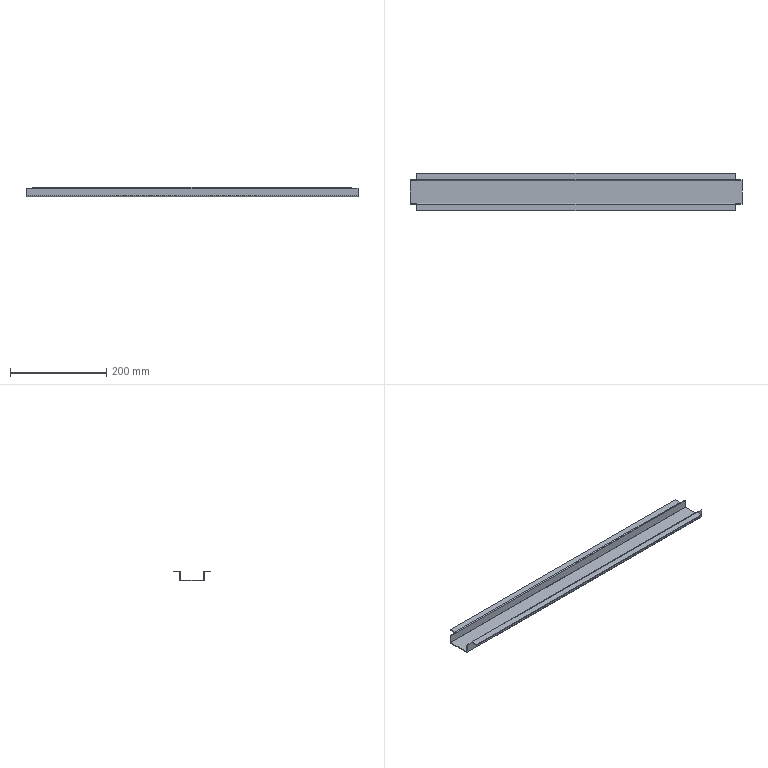Part | STEP file | FHD-021-001-T rack welded part T | 1 solid | 30 faces | box 690 x 77 x 20 mm | volume 115059 mm3 | plane 22 | cylinder 8 | commonest cylinder face diameters 0.4 x4 3.4 x4